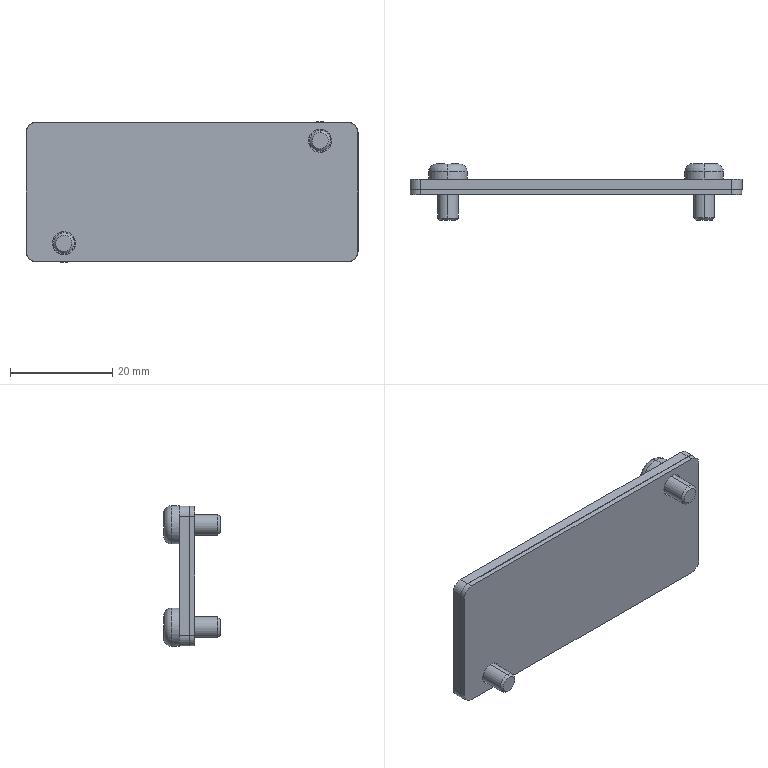Part | SolidWorks | features BaseBody 1 | 1 solid | 81 faces | box 64.8 x 11 x 27.5 mm | volume 5589 mm3 | plane 43 | cylinder 30 | cone 4 | torus 4 | commonest cylinder face diameters 4 x12 5.143 x10 4.5 x4 7.5 x4